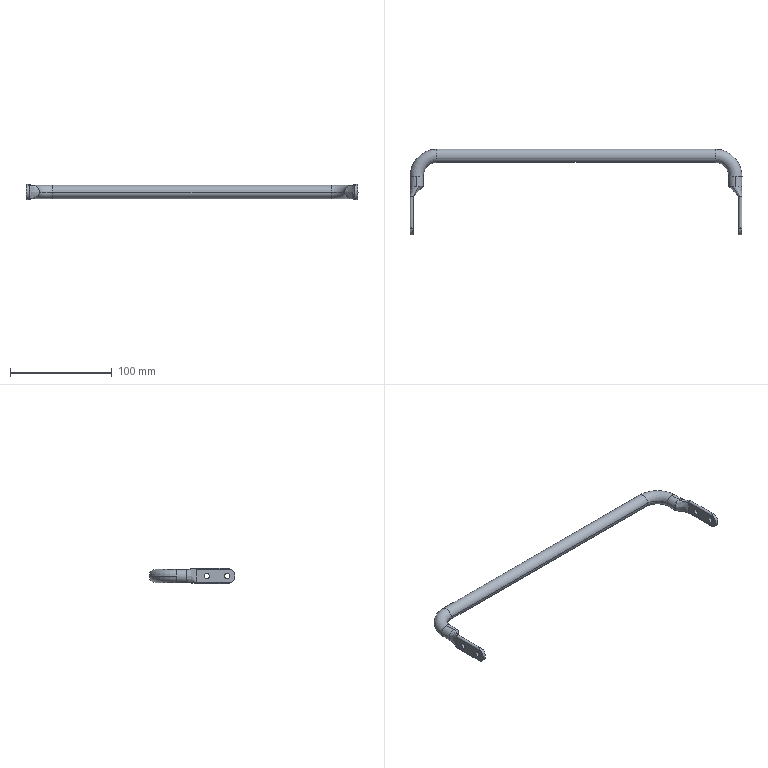Part | SolidWorks | features BaseBody 1 | 1 solid | 44 faces | box 326 x 84 x 15.001 mm | volume 17967 mm3 | cylinder 26 | torus 8 | plane 6 | spline 4 | commonest cylinder face diameters 5.2 x8 11 x6 13 x6 3 x4 15 x2